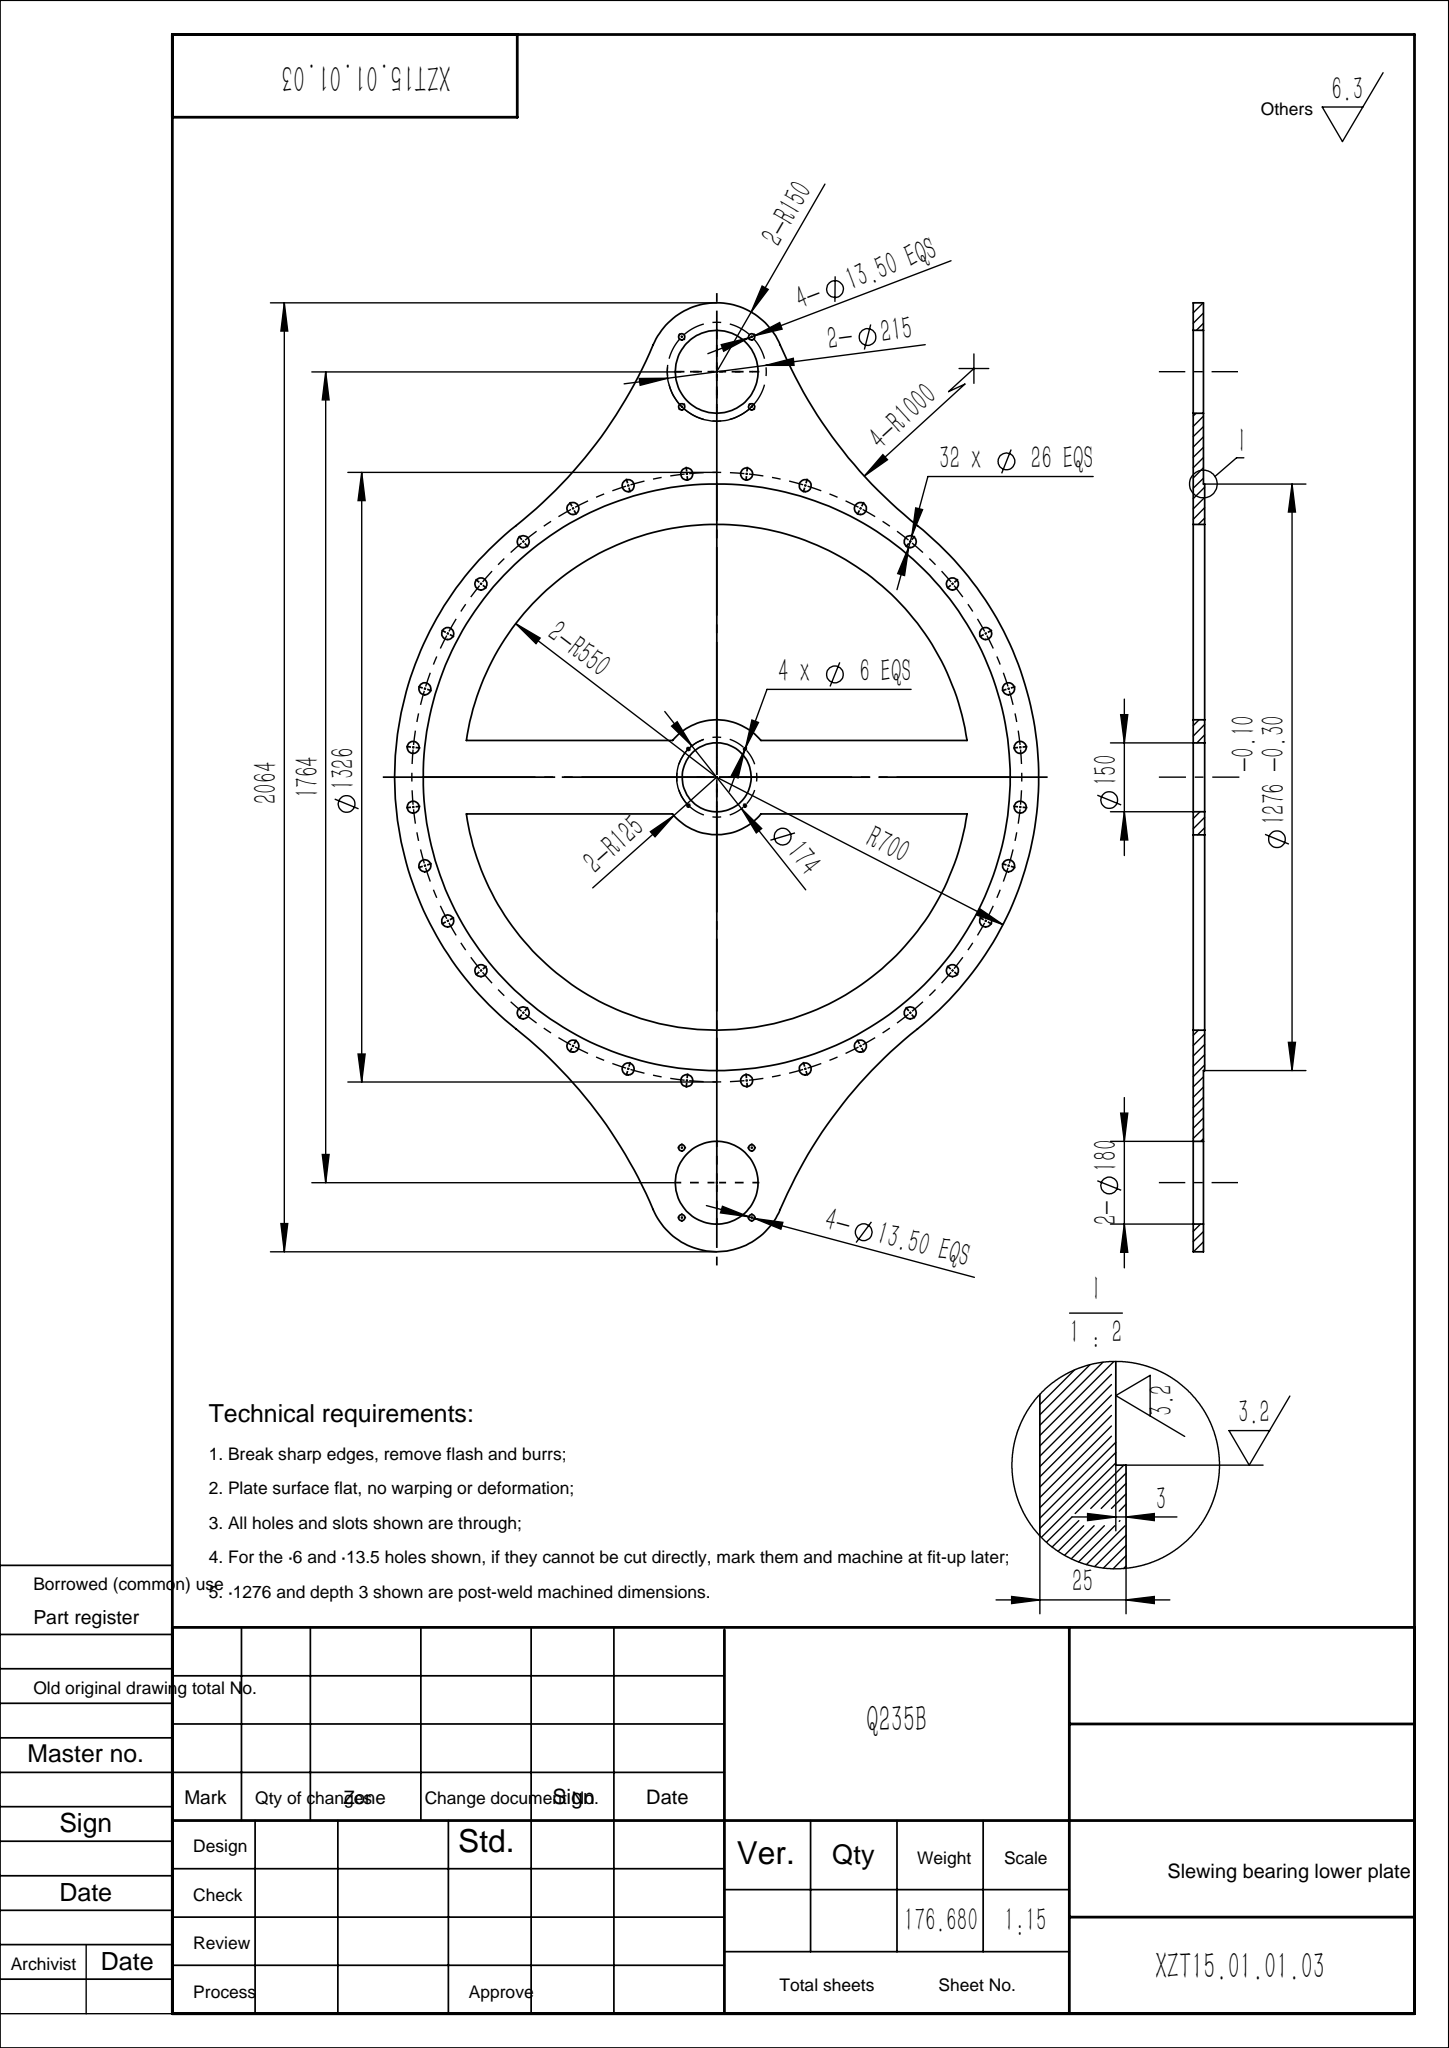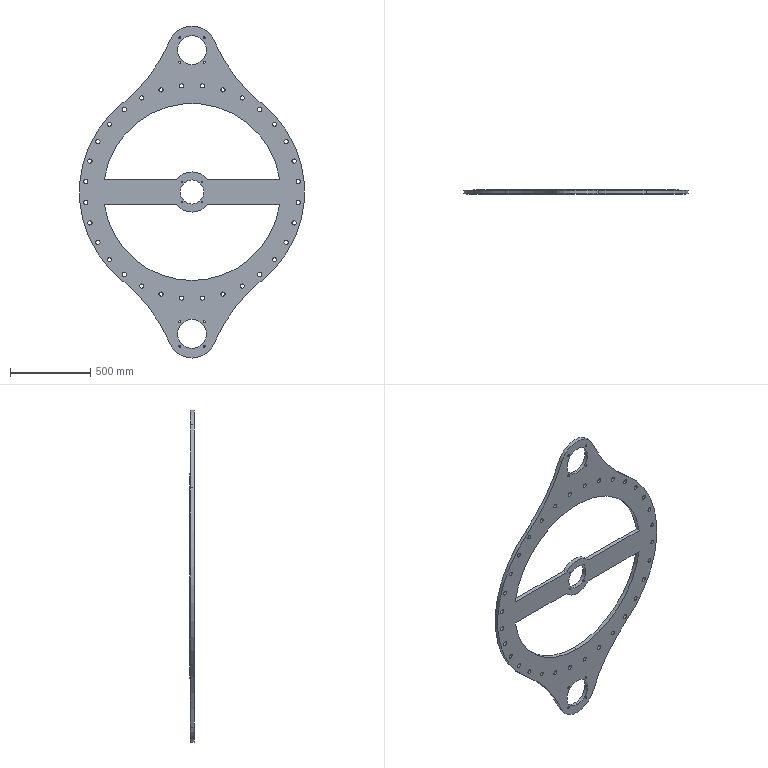Part | SolidWorks | features HoleWzd 3, Extrusion 1, ICE 1, MirrorPattern 1 | 1 solid | 118 faces | box 1400 x 25 x 2064 mm | volume 22506945 mm3 | cylinder 111 | plane 7 | commonest cylinder face diameters 26 x64 13.5 x16 6 x8 180 x4 2000 x4 250 x3